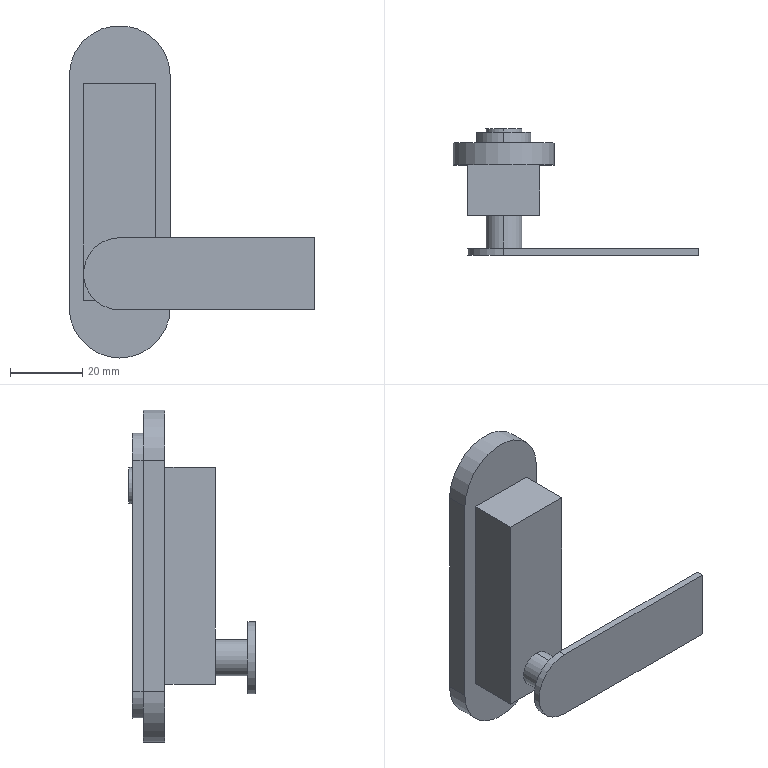Part | STEP file | Door lock KL-MS77-1001 | 1 solid | 34 faces | box 68 x 35 x 92 mm | volume 37880 mm3 | plane 23 | cylinder 11 | commonest cylinder face diameters 10 x4 15 x3 28 x3 20 x1